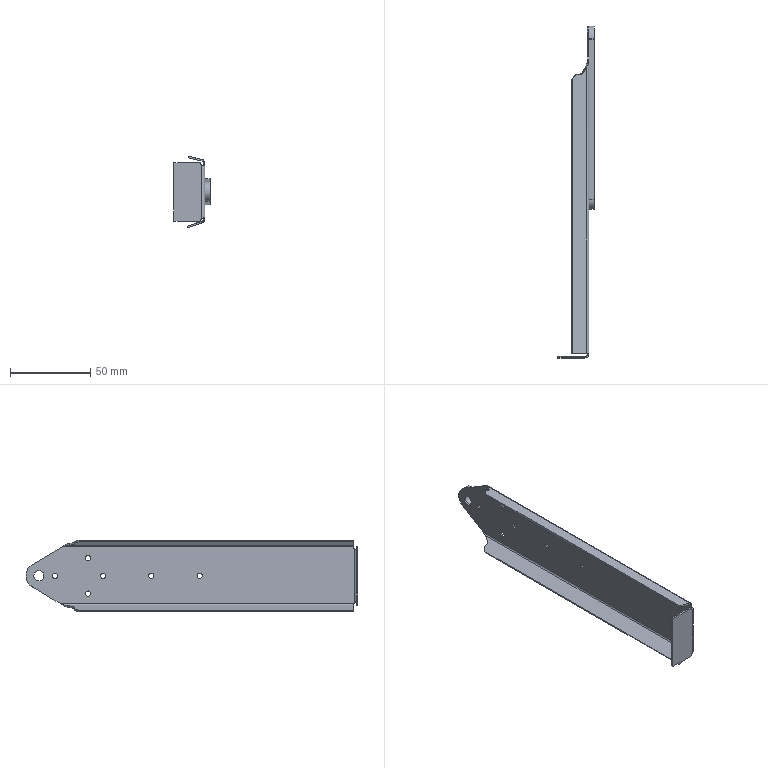Part | SolidWorks | features BaseBody 2 | 2 solids | 74 faces | box 22.422 x 206.422 x 44.537 mm | volume 16293 mm3 | cylinder 41 | plane 27 | spline 6 | commonest cylinder face diameters 3.2 x20 4 x7 6.35 x4 16 x4 2 x3 5 x2